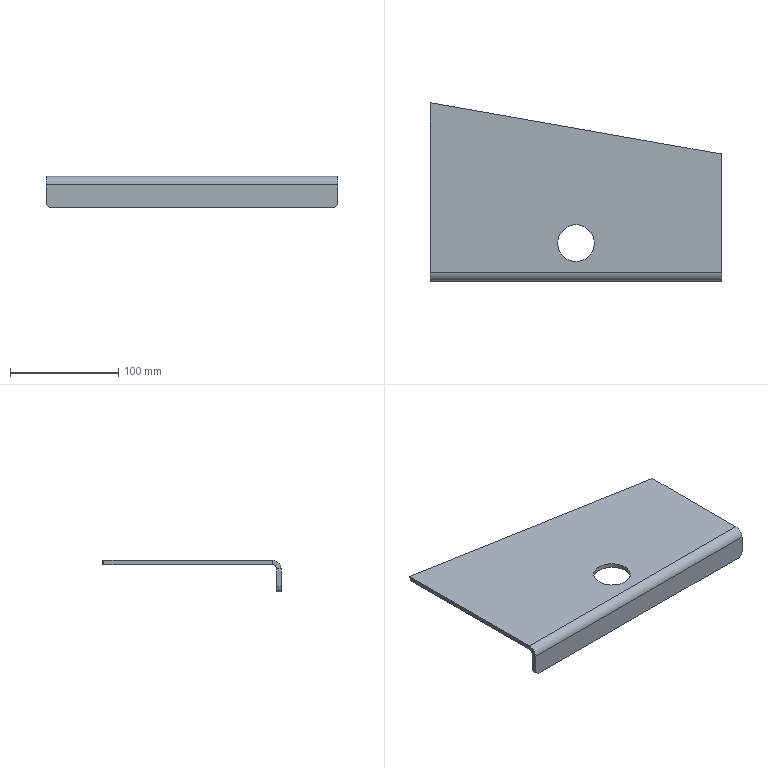Part | STEP file | 001-011-Blanking flip vertical plate | 1 solid | 20 faces | box 270 x 164.808 x 29 mm | volume 173034 mm3 | plane 12 | cylinder 8 | commonest cylinder face diameters 2 x2 10 x2 34 x2 8 x1 16 x1
STEP:
#1=CARTESIAN_POINT('',(0.,0.,0.));
#2=DIRECTION('',(0.,0.,1.));
#3=DIRECTION('',(1.,0.,0.));
#4=AXIS2_PLACEMENT_3D('',#1,#2,#3);
#5=CARTESIAN_POINT('',(-17.,-47.5,0.));
#6=VERTEX_POINT('',#5);
#7=CARTESIAN_POINT('',(-17.,-47.5,-4.));
#8=VERTEX_POINT('',#7);
#9=CARTESIAN_POINT('',(-17.,-47.5,0.));
#10=DIRECTION('',(0.,0.,-1.));
#11=VECTOR('',#10,1.);
#12=LINE('',#9,#11);
#13=CARTESIAN_POINT('',(0.,-47.5,0.));
#14=DIRECTION('',(0.,0.,-1.));
#15=DIRECTION('',(-1.,0.,0.));
#16=AXIS2_PLACEMENT_3D('',#13,#14,#15);
#17=CYLINDRICAL_SURFACE('',#16,17.);
#18=CARTESIAN_POINT('',(6.283,0.));
#19=DIRECTION('',(0.,1.));
#20=VECTOR('',#19,1.);
#21=LINE('',#18,#20);
#22=(GEOMETRIC_REPRESENTATION_CONTEXT(2)PARAMETRIC_REPRESENTATION_CONTEXT()REPRESENTATION_CONTEXT('',''));
#23=DEFINITIONAL_REPRESENTATION('',(#21),#22);
#24=PCURVE('',#17,#23);
#25=CARTESIAN_POINT('',(0.,-47.5,0.));
#26=DIRECTION('',(0.,0.,-1.));
#27=DIRECTION('',(-1.,0.,0.));
#28=AXIS2_PLACEMENT_3D('',#25,#26,#27);
#29=CYLINDRICAL_SURFACE('',#28,17.);
#30=CARTESIAN_POINT('',(0.,0.));
#31=DIRECTION('',(0.,1.));
#32=VECTOR('',#31,1.);
#33=LINE('',#30,#32);
#34=(GEOMETRIC_REPRESENTATION_CONTEXT(2)PARAMETRIC_REPRESENTATION_CONTEXT()REPRESENTATION_CONTEXT('',''));
#35=DEFINITIONAL_REPRESENTATION('',(#33),#34);
#36=PCURVE('',#29,#35);
#37=SURFACE_CURVE('',#12,(#24,#36),.PCURVE_S1.);
#38=EDGE_CURVE('',#6,#8,#37,.T.);
#39=ORIENTED_EDGE('',*,*,#38,.T.);
#40=CARTESIAN_POINT('',(17.,-47.5,-4.));
#41=VERTEX_POINT('',#40);
#42=CARTESIAN_POINT('',(0.,-47.5,-4.));
#43=DIRECTION('',(0.,0.,-1.));
#44=DIRECTION('',(-1.,0.,0.));
#45=AXIS2_PLACEMENT_3D('',#42,#43,#44);
#46=CIRCLE('',#45,17.);
#47=CARTESIAN_POINT('',(0.,4.));
#48=DIRECTION('',(1.,0.));
#49=VECTOR('',#48,1.);
#50=LINE('',#47,#49);
#51=(GEOMETRIC_REPRESENTATION_CONTEXT(2)PARAMETRIC_REPRESENTATION_CONTEXT()REPRESENTATION_CONTEXT('',''));
#52=DEFINITIONAL_REPRESENTATION('',(#50),#51);
#53=PCURVE('',#17,#52);
#54=CARTESIAN_POINT('',(0.,0.,-4.));
#55=DIRECTION('',(0.,0.,-1.));
#56=DIRECTION('',(-1.,0.,0.));
#57=AXIS2_PLACEMENT_3D('',#54,#55,#56);
#58=PLANE('',#57);
#59=CARTESIAN_POINT('',(0.,-47.5));
#60=DIRECTION('',(1.,0.));
#61=AXIS2_PLACEMENT_2D('',#59,#60);
#62=CIRCLE('',#61,17.);
#63=(GEOMETRIC_REPRESENTATION_CONTEXT(2)PARAMETRIC_REPRESENTATION_CONTEXT()REPRESENTATION_CONTEXT('',''));
#64=DEFINITIONAL_REPRESENTATION('',(#62),#63);
#65=PCURVE('',#58,#64);
#66=SURFACE_CURVE('',#46,(#53,#65),.PCURVE_S1.);
#67=EDGE_CURVE('',#41,#8,#66,.T.);
#68=ORIENTED_EDGE('',*,*,#67,.F.);
#69=CARTESIAN_POINT('',(17.,-47.5,0.));
#70=VERTEX_POINT('',#69);
#71=CARTESIAN_POINT('',(17.,-47.5,0.));
#72=DIRECTION('',(0.,0.,-1.));
#73=VECTOR('',#72,1.);
#74=LINE('',#71,#73);
#75=CARTESIAN_POINT('',(3.142,0.));
#76=DIRECTION('',(0.,1.));
#77=VECTOR('',#76,1.);
#78=LINE('',#75,#77);
#79=(GEOMETRIC_REPRESENTATION_CONTEXT(2)PARAMETRIC_REPRESENTATION_CONTEXT()REPRESENTATION_CONTEXT('',''));
#80=DEFINITIONAL_REPRESENTATION('',(#78),#79);
#81=PCURVE('',#17,#80);
#82=CARTESIAN_POINT('',(3.142,0.));
#83=DIRECTION('',(0.,1.));
#84=VECTOR('',#83,1.);
#85=LINE('',#82,#84);
#86=(GEOMETRIC_REPRESENTATION_CONTEXT(2)PARAMETRIC_REPRESENTATION_CONTEXT()REPRESENTATION_CONTEXT('',''));
#87=DEFINITIONAL_REPRESENTATION('',(#85),#86);
#88=PCURVE('',#29,#87);
#89=SURFACE_CURVE('',#74,(#81,#88),.PCURVE_S1.);
#90=EDGE_CURVE('',#70,#41,#89,.T.);
#91=ORIENTED_EDGE('',*,*,#90,.F.);
#92=CARTESIAN_POINT('',(0.,-47.5,0.));
#93=DIRECTION('',(0.,0.,-1.));
#94=DIRECTION('',(-1.,0.,0.));
#95=AXIS2_PLACEMENT_3D('',#92,#93,#94);
#96=CIRCLE('',#95,17.);
#97=CARTESIAN_POINT('',(0.,0.));
#98=DIRECTION('',(1.,0.));
#99=VECTOR('',#98,1.);
#100=LINE('',#97,#99);
#101=(GEOMETRIC_REPRESENTATION_CONTEXT(2)PARAMETRIC_REPRESENTATION_CONTEXT()REPRESENTATION_CONTEXT('',''));
#102=DEFINITIONAL_REPRESENTATION('',(#100),#101);
#103=PCURVE('',#17,#102);
#104=CARTESIAN_POINT('',(0.,0.,0.));
#105=DIRECTION('',(0.,0.,-1.));
#106=DIRECTION('',(-1.,0.,0.));
#107=AXIS2_PLACEMENT_3D('',#104,#105,#106);
#108=PLANE('',#107);
#109=CARTESIAN_POINT('',(0.,-47.5));
#110=DIRECTION('',(1.,0.));
#111=AXIS2_PLACEMENT_2D('',#109,#110);
#112=CIRCLE('',#111,17.);
#113=(GEOMETRIC_REPRESENTATION_CONTEXT(2)PARAMETRIC_REPRESENTATION_CONTEXT()REPRESENTATION_CONTEXT('',''));
#114=DEFINITIONAL_REPRESENTATION('',(#112),#113);
#115=PCURVE('',#108,#114);
#116=SURFACE_CURVE('',#96,(#103,#115),.PCURVE_S1.);
#117=EDGE_CURVE('',#70,#6,#116,.T.);
#118=ORIENTED_EDGE('',*,*,#117,.T.);
#119=EDGE_LOOP('',(#39,#68,#91,#118));
#120=FACE_BOUND('',#119,.F.);
#121=ADVANCED_FACE('',(#120),#17,.F.);
#122=CARTESIAN_POINT('',(-135.,81.308,0.));
#123=VERTEX_POINT('',#122);
#124=CARTESIAN_POINT('',(-135.,-74.5,0.));
#125=VERTEX_POINT('',#124);
#126=CARTESIAN_POINT('',(-135.,-82.5,0.));
#127=DIRECTION('',(0.,-1.,0.));
#128=VECTOR('',#127,1.);
#129=LINE('',#126,#128);
#130=CARTESIAN_POINT('',(-135.,-82.5,-4.));
#131=DIRECTION('',(-1.,0.,0.));
#132=DIRECTION('',(0.,0.,1.));
#133=AXIS2_PLACEMENT_3D('',#130,#131,#132);
#134=PLANE('',#133);
#135=CARTESIAN_POINT('',(4.,0.));
#136=DIRECTION('',(0.,-1.));
#137=VECTOR('',#136,1.);
#138=LINE('',#135,#137);
#139=(GEOMETRIC_REPRESENTATION_CONTEXT(2)PARAMETRIC_REPRESENTATION_CONTEXT()REPRESENTATION_CONTEXT('',''));
#140=DEFINITIONAL_REPRESENTATION('',(#138),#139);
#141=PCURVE('',#134,#140);
#142=CARTESIAN_POINT('',(135.,-82.5));
#143=DIRECTION('',(0.,-1.));
#144=VECTOR('',#143,1.);
#145=LINE('',#142,#144);
#146=(GEOMETRIC_REPRESENTATION_CONTEXT(2)PARAMETRIC_REPRESENTATION_CONTEXT()REPRESENTATION_CONTEXT('',''));
#147=DEFINITIONAL_REPRESENTATION('',(#145),#146);
#148=PCURVE('',#108,#147);
#149=SURFACE_CURVE('',#129,(#141,#148),.PCURVE_S1.);
#150=EDGE_CURVE('',#123,#125,#149,.T.);
#151=ORIENTED_EDGE('',*,*,#150,.F.);
#152=CARTESIAN_POINT('',(-135.,81.308,-4.));
#153=VERTEX_POINT('',#152);
#154=CARTESIAN_POINT('',(-135.,81.308,-4.));
#155=DIRECTION('',(0.,0.,-1.));
#156=VECTOR('',#155,1.);
#157=LINE('',#154,#156);
#158=CARTESIAN_POINT('',(0.,163.808));
#159=DIRECTION('',(-1.,0.));
#160=VECTOR('',#159,1.);
#161=LINE('',#158,#160);
#162=(GEOMETRIC_REPRESENTATION_CONTEXT(2)PARAMETRIC_REPRESENTATION_CONTEXT()REPRESENTATION_CONTEXT('',''));
#163=DEFINITIONAL_REPRESENTATION('',(#161),#162);
#164=PCURVE('',#134,#163);
#165=CARTESIAN_POINT('',(-134.,81.308,-29.));
#166=DIRECTION('',(0.,0.,-1.));
#167=DIRECTION('',(-1.,0.,0.));
#168=AXIS2_PLACEMENT_3D('',#165,#166,#167);
#169=CYLINDRICAL_SURFACE('',#168,1.);
#170=CARTESIAN_POINT('',(0.,-25.));
#171=DIRECTION('',(0.,1.));
#172=VECTOR('',#171,1.);
#173=LINE('',#170,#172);
#174=(GEOMETRIC_REPRESENTATION_CONTEXT(2)PARAMETRIC_REPRESENTATION_CONTEXT()REPRESENTATION_CONTEXT('',''));
#175=DEFINITIONAL_REPRESENTATION('',(#173),#174);
#176=PCURVE('',#169,#175);
#177=SURFACE_CURVE('',#157,(#164,#176),.PCURVE_S1.);
#178=EDGE_CURVE('',#123,#153,#177,.T.);
#179=ORIENTED_EDGE('',*,*,#178,.T.);
#180=CARTESIAN_POINT('',(-135.,-74.5,-4.));
#181=VERTEX_POINT('',#180);
#182=CARTESIAN_POINT('',(-135.,-82.5,-4.));
#183=DIRECTION('',(0.,-1.,0.));
#184=VECTOR('',#183,1.);
#185=LINE('',#182,#184);
#186=CARTESIAN_POINT('',(0.,0.));
#187=DIRECTION('',(0.,-1.));
#188=VECTOR('',#187,1.);
#189=LINE('',#186,#188);
#190=(GEOMETRIC_REPRESENTATION_CONTEXT(2)PARAMETRIC_REPRESENTATION_CONTEXT()REPRESENTATION_CONTEXT('',''));
#191=DEFINITIONAL_REPRESENTATION('',(#189),#190);
#192=PCURVE('',#134,#191);
#193=CARTESIAN_POINT('',(135.,-82.5));
#194=DIRECTION('',(0.,-1.));
#195=VECTOR('',#194,1.);
#196=LINE('',#193,#195);
#197=(GEOMETRIC_REPRESENTATION_CONTEXT(2)PARAMETRIC_REPRESENTATION_CONTEXT()REPRESENTATION_CONTEXT('',''));
#198=DEFINITIONAL_REPRESENTATION('',(#196),#197);
#199=PCURVE('',#58,#198);
#200=SURFACE_CURVE('',#185,(#192,#199),.PCURVE_S1.);
#201=EDGE_CURVE('',#153,#181,#200,.T.);
#202=ORIENTED_EDGE('',*,*,#201,.T.);
#203=CARTESIAN_POINT('',(-135.,-74.5,-4.));
#204=DIRECTION('',(0.,0.,1.));
#205=VECTOR('',#204,1.);
#206=LINE('',#203,#205);
#207=CARTESIAN_POINT('',(0.,8.));
#208=DIRECTION('',(1.,0.));
#209=VECTOR('',#208,1.);
#210=LINE('',#207,#209);
#211=(GEOMETRIC_REPRESENTATION_CONTEXT(2)PARAMETRIC_REPRESENTATION_CONTEXT()REPRESENTATION_CONTEXT('',''));
#212=DEFINITIONAL_REPRESENTATION('',(#210),#211);
#213=PCURVE('',#134,#212);
#214=CARTESIAN_POINT('',(-135.,-74.5,-8.));
#215=DIRECTION('',(1.,0.,0.));
#216=DIRECTION('',(0.,0.,-1.));
#217=AXIS2_PLACEMENT_3D('',#214,#215,#216);
#218=PLANE('',#217);
#219=CARTESIAN_POINT('',(-4.,0.));
#220=DIRECTION('',(-1.,0.));
#221=VECTOR('',#220,1.);
#222=LINE('',#219,#221);
#223=(GEOMETRIC_REPRESENTATION_CONTEXT(2)PARAMETRIC_REPRESENTATION_CONTEXT()REPRESENTATION_CONTEXT('',''));
#224=DEFINITIONAL_REPRESENTATION('',(#222),#223);
#225=PCURVE('',#218,#224);
#226=SURFACE_CURVE('',#206,(#213,#225),.PCURVE_S1.);
#227=EDGE_CURVE('',#181,#125,#226,.T.);
#228=ORIENTED_EDGE('',*,*,#227,.T.);
#229=EDGE_LOOP('',(#151,#179,#202,#228));
#230=FACE_BOUND('',#229,.T.);
#231=ADVANCED_FACE('',(#230),#134,.T.);
#232=CARTESIAN_POINT('',(0.,-47.5,-4.));
#233=DIRECTION('',(0.,0.,-1.));
#234=DIRECTION('',(-1.,0.,0.));
#235=AXIS2_PLACEMENT_3D('',#232,#233,#234);
#236=CIRCLE('',#235,17.);
#237=CARTESIAN_POINT('',(0.,-47.5));
#238=DIRECTION('',(1.,0.));
#239=AXIS2_PLACEMENT_2D('',#237,#238);
#240=CIRCLE('',#239,17.);
#241=(GEOMETRIC_REPRESENTATION_CONTEXT(2)PARAMETRIC_REPRESENTATION_CONTEXT()REPRESENTATION_CONTEXT('',''));
#242=DEFINITIONAL_REPRESENTATION('',(#240),#241);
#243=PCURVE('',#58,#242);
#244=CARTESIAN_POINT('',(0.,4.));
#245=DIRECTION('',(1.,0.));
#246=VECTOR('',#245,1.);
#247=LINE('',#244,#246);
#248=(GEOMETRIC_REPRESENTATION_CONTEXT(2)PARAMETRIC_REPRESENTATION_CONTEXT()REPRESENTATION_CONTEXT('',''));
#249=DEFINITIONAL_REPRESENTATION('',(#247),#248);
#250=PCURVE('',#29,#249);
#251=SURFACE_CURVE('',#236,(#243,#250),.PCURVE_S1.);
#252=EDGE_CURVE('',#8,#41,#251,.T.);
#253=ORIENTED_EDGE('',*,*,#252,.F.);
#254=ORIENTED_EDGE('',*,*,#67,.F.);
#255=EDGE_LOOP('',(#253,#254));
#256=FACE_BOUND('',#255,.T.);
#257=ORIENTED_EDGE('',*,*,#201,.F.);
#258=CARTESIAN_POINT('',(-133.826,82.293,-4.));
#259=VERTEX_POINT('',#258);
#260=CARTESIAN_POINT('',(-134.,81.308,-4.));
#261=DIRECTION('',(0.,0.,-1.));
#262=DIRECTION('',(-1.,0.,0.));
#263=AXIS2_PLACEMENT_3D('',#260,#261,#262);
#264=CIRCLE('',#263,1.);
#265=CARTESIAN_POINT('',(134.,81.308));
#266=DIRECTION('',(1.,0.));
#267=AXIS2_PLACEMENT_2D('',#265,#266);
#268=CIRCLE('',#267,1.);
#269=(GEOMETRIC_REPRESENTATION_CONTEXT(2)PARAMETRIC_REPRESENTATION_CONTEXT()REPRESENTATION_CONTEXT('',''));
#270=DEFINITIONAL_REPRESENTATION('',(#268),#269);
#271=PCURVE('',#58,#270);
#272=CARTESIAN_POINT('',(0.,-25.));
#273=DIRECTION('',(1.,0.));
#274=VECTOR('',#273,1.);
#275=LINE('',#272,#274);
#276=(GEOMETRIC_REPRESENTATION_CONTEXT(2)PARAMETRIC_REPRESENTATION_CONTEXT()REPRESENTATION_CONTEXT('',''));
#277=DEFINITIONAL_REPRESENTATION('',(#275),#276);
#278=PCURVE('',#169,#277);
#279=SURFACE_CURVE('',#264,(#271,#278),.PCURVE_S1.);
#280=EDGE_CURVE('',#153,#259,#279,.T.);
#281=ORIENTED_EDGE('',*,*,#280,.T.);
#282=CARTESIAN_POINT('',(134.174,35.037,-4.));
#283=VERTEX_POINT('',#282);
#284=CARTESIAN_POINT('',(10.038,56.926,-4.));
#285=DIRECTION('',(-0.9848,0.1736,0.));
#286=VECTOR('',#285,1.);
#287=LINE('',#284,#286);
#288=CARTESIAN_POINT('',(-10.038,56.926));
#289=DIRECTION('',(0.9848,0.1736));
#290=VECTOR('',#289,1.);
#291=LINE('',#288,#290);
#292=(GEOMETRIC_REPRESENTATION_CONTEXT(2)PARAMETRIC_REPRESENTATION_CONTEXT()REPRESENTATION_CONTEXT('',''));
#293=DEFINITIONAL_REPRESENTATION('',(#291),#292);
#294=PCURVE('',#58,#293);
#295=CARTESIAN_POINT('',(135.,34.892,-29.));
#296=DIRECTION('',(-0.1736,-0.9848,0.));
#297=DIRECTION('',(0.9848,-0.1736,0.));
#298=AXIS2_PLACEMENT_3D('',#295,#296,#297);
#299=PLANE('',#298);
#300=CARTESIAN_POINT('',(-126.89,25.));
#301=DIRECTION('',(-1.,0.));
#302=VECTOR('',#301,1.);
#303=LINE('',#300,#302);
#304=(GEOMETRIC_REPRESENTATION_CONTEXT(2)PARAMETRIC_REPRESENTATION_CONTEXT()REPRESENTATION_CONTEXT('',''));
#305=DEFINITIONAL_REPRESENTATION('',(#303),#304);
#306=PCURVE('',#299,#305);
#307=SURFACE_CURVE('',#287,(#294,#306),.PCURVE_S1.);
#308=EDGE_CURVE('',#283,#259,#307,.T.);
#309=ORIENTED_EDGE('',*,*,#308,.F.);
#310=CARTESIAN_POINT('',(135.,34.053,-4.));
#311=VERTEX_POINT('',#310);
#312=CARTESIAN_POINT('',(134.,34.053,-4.));
#313=DIRECTION('',(0.,0.,-1.));
#314=DIRECTION('',(-1.,0.,0.));
#315=AXIS2_PLACEMENT_3D('',#312,#313,#314);
#316=CIRCLE('',#315,1.);
#317=CARTESIAN_POINT('',(-134.,34.053));
#318=DIRECTION('',(1.,0.));
#319=AXIS2_PLACEMENT_2D('',#317,#318);
#320=CIRCLE('',#319,1.);
#321=(GEOMETRIC_REPRESENTATION_CONTEXT(2)PARAMETRIC_REPRESENTATION_CONTEXT()REPRESENTATION_CONTEXT('',''));
#322=DEFINITIONAL_REPRESENTATION('',(#320),#321);
#323=PCURVE('',#58,#322);
#324=CARTESIAN_POINT('',(134.,34.053,-4.));
#325=DIRECTION('',(0.,0.,-1.));
#326=DIRECTION('',(-1.,0.,0.));
#327=AXIS2_PLACEMENT_3D('',#324,#325,#326);
#328=CYLINDRICAL_SURFACE('',#327,1.);
#329=CARTESIAN_POINT('',(0.,0.));
#330=DIRECTION('',(1.,0.));
#331=VECTOR('',#330,1.);
#332=LINE('',#329,#331);
#333=(GEOMETRIC_REPRESENTATION_CONTEXT(2)PARAMETRIC_REPRESENTATION_CONTEXT()REPRESENTATION_CONTEXT('',''));
#334=DEFINITIONAL_REPRESENTATION('',(#332),#333);
#335=PCURVE('',#328,#334);
#336=SURFACE_CURVE('',#316,(#323,#335),.PCURVE_S1.);
#337=EDGE_CURVE('',#283,#311,#336,.T.);
#338=ORIENTED_EDGE('',*,*,#337,.T.);
#339=CARTESIAN_POINT('',(135.,-74.5,-4.));
#340=VERTEX_POINT('',#339);
#341=CARTESIAN_POINT('',(135.,-82.5,-4.));
#342=DIRECTION('',(0.,1.,0.));
#343=VECTOR('',#342,1.);
#344=LINE('',#341,#343);
#345=CARTESIAN_POINT('',(-135.,-82.5));
#346=DIRECTION('',(0.,1.));
#347=VECTOR('',#346,1.);
#348=LINE('',#345,#347);
#349=(GEOMETRIC_REPRESENTATION_CONTEXT(2)PARAMETRIC_REPRESENTATION_CONTEXT()REPRESENTATION_CONTEXT('',''));
#350=DEFINITIONAL_REPRESENTATION('',(#348),#349);
#351=PCURVE('',#58,#350);
#352=CARTESIAN_POINT('',(135.,-82.5,-4.));
#353=DIRECTION('',(1.,0.,0.));
#354=DIRECTION('',(0.,1.,0.));
#355=AXIS2_PLACEMENT_3D('',#352,#353,#354);
#356=PLANE('',#355);
#357=CARTESIAN_POINT('',(0.,0.));
#358=DIRECTION('',(1.,0.));
#359=VECTOR('',#358,1.);
#360=LINE('',#357,#359);
#361=(GEOMETRIC_REPRESENTATION_CONTEXT(2)PARAMETRIC_REPRESENTATION_CONTEXT()REPRESENTATION_CONTEXT('',''));
#362=DEFINITIONAL_REPRESENTATION('',(#360),#361);
#363=PCURVE('',#356,#362);
#364=SURFACE_CURVE('',#344,(#351,#363),.PCURVE_S1.);
#365=EDGE_CURVE('',#340,#311,#364,.T.);
#366=ORIENTED_EDGE('',*,*,#365,.F.);
#367=CARTESIAN_POINT('',(-135.,-74.5,-4.));
#368=DIRECTION('',(1.,0.,0.));
#369=VECTOR('',#368,1.);
#370=LINE('',#367,#369);
#371=CARTESIAN_POINT('',(135.,-74.5));
#372=DIRECTION('',(-1.,0.));
#373=VECTOR('',#372,1.);
#374=LINE('',#371,#373);
#375=(GEOMETRIC_REPRESENTATION_CONTEXT(2)PARAMETRIC_REPRESENTATION_CONTEXT()REPRESENTATION_CONTEXT('',''));
#376=DEFINITIONAL_REPRESENTATION('',(#374),#375);
#377=PCURVE('',#58,#376);
#378=CARTESIAN_POINT('',(-135.,-74.5,-8.));
#379=DIRECTION('',(-1.,0.,0.));
#380=DIRECTION('',(0.,-1.,0.));
#381=AXIS2_PLACEMENT_3D('',#378,#379,#380);
#382=CYLINDRICAL_SURFACE('',#381,4.);
#383=CARTESIAN_POINT('',(1.571,0.));
#384=DIRECTION('',(0.,-1.));
#385=VECTOR('',#384,1.);
#386=LINE('',#383,#385);
#387=(GEOMETRIC_REPRESENTATION_CONTEXT(2)PARAMETRIC_REPRESENTATION_CONTEXT()REPRESENTATION_CONTEXT('',''));
#388=DEFINITIONAL_REPRESENTATION('',(#386),#387);
#389=PCURVE('',#382,#388);
#390=SURFACE_CURVE('',#370,(#377,#389),.PCURVE_S1.);
#391=EDGE_CURVE('',#181,#340,#390,.T.);
#392=ORIENTED_EDGE('',*,*,#391,.F.);
#393=EDGE_LOOP('',(#257,#281,#309,#338,#366,#392));
#394=FACE_BOUND('',#393,.T.);
#395=ADVANCED_FACE('',(#256,#394),#58,.T.);
#396=CARTESIAN_POINT('',(0.,-47.5,0.));
#397=DIRECTION('',(0.,0.,-1.));
#398=DIRECTION('',(-1.,0.,0.));
#399=AXIS2_PLACEMENT_3D('',#396,#397,#398);
#400=CIRCLE('',#399,17.);
#401=CARTESIAN_POINT('',(0.,-47.5));
#402=DIRECTION('',(1.,0.));
#403=AXIS2_PLACEMENT_2D('',#401,#402);
#404=CIRCLE('',#403,17.);
#405=(GEOMETRIC_REPRESENTATION_CONTEXT(2)PARAMETRIC_REPRESENTATION_CONTEXT()REPRESENTATION_CONTEXT('',''));
#406=DEFINITIONAL_REPRESENTATION('',(#404),#405);
#407=PCURVE('',#108,#406);
#408=CARTESIAN_POINT('',(0.,0.));
#409=DIRECTION('',(1.,0.));
#410=VECTOR('',#409,1.);
#411=LINE('',#408,#410);
#412=(GEOMETRIC_REPRESENTATION_CONTEXT(2)PARAMETRIC_REPRESENTATION_CONTEXT()REPRESENTATION_CONTEXT('',''));
#413=DEFINITIONAL_REPRESENTATION('',(#411),#412);
#414=PCURVE('',#29,#413);
#415=SURFACE_CURVE('',#400,(#407,#414),.PCURVE_S1.);
#416=EDGE_CURVE('',#6,#70,#415,.T.);
#417=ORIENTED_EDGE('',*,*,#416,.T.);
#418=ORIENTED_EDGE('',*,*,#117,.T.);
#419=EDGE_LOOP('',(#417,#418));
#420=FACE_BOUND('',#419,.T.);
#421=CARTESIAN_POINT('',(-133.826,82.293,0.));
#422=VERTEX_POINT('',#421);
#423=CARTESIAN_POINT('',(134.174,35.037,0.));
#424=VERTEX_POINT('',#423);
#425=CARTESIAN_POINT('',(135.,34.892,0.));
#426=DIRECTION('',(0.9848,-0.1736,0.));
#427=VECTOR('',#426,1.);
#428=LINE('',#425,#427);
#429=CARTESIAN_POINT('',(-135.,34.892));
#430=DIRECTION('',(-0.9848,-0.1736));
#431=VECTOR('',#430,1.);
#432=LINE('',#429,#431);
#433=(GEOMETRIC_REPRESENTATION_CONTEXT(2)PARAMETRIC_REPRESENTATION_CONTEXT()REPRESENTATION_CONTEXT('',''));
#434=DEFINITIONAL_REPRESENTATION('',(#432),#433);
#435=PCURVE('',#108,#434);
#436=CARTESIAN_POINT('',(0.,29.));
#437=DIRECTION('',(1.,0.));
#438=VECTOR('',#437,1.);
#439=LINE('',#436,#438);
#440=(GEOMETRIC_REPRESENTATION_CONTEXT(2)PARAMETRIC_REPRESENTATION_CONTEXT()REPRESENTATION_CONTEXT('',''));
#441=DEFINITIONAL_REPRESENTATION('',(#439),#440);
#442=PCURVE('',#299,#441);
#443=SURFACE_CURVE('',#428,(#435,#442),.PCURVE_S1.);
#444=EDGE_CURVE('',#422,#424,#443,.T.);
#445=ORIENTED_EDGE('',*,*,#444,.F.);
#446=CARTESIAN_POINT('',(-134.,81.308,0.));
#447=DIRECTION('',(0.,0.,1.));
#448=DIRECTION('',(-1.,0.,0.));
#449=AXIS2_PLACEMENT_3D('',#446,#447,#448);
#450=CIRCLE('',#449,1.);
#451=CARTESIAN_POINT('',(135.,81.308));
#452=CARTESIAN_POINT('',(135.,79.576));
#453=CARTESIAN_POINT('',(133.5,80.442));
#454=CARTESIAN_POINT('',(132.,81.308));
#455=CARTESIAN_POINT('',(133.5,82.174));
#456=CARTESIAN_POINT('',(135.,83.04));
#457=CARTESIAN_POINT('',(135.,81.308));
#458=(BOUNDED_CURVE()B_SPLINE_CURVE(2,(#451,#452,#453,#454,#455,#456,#457),.UNSPECIFIED.,.T.,.F.)B_SPLINE_CURVE_WITH_KNOTS((1,2,2,2,2,1),(-2.094,0.,2.094,4.189,6.283,8.378),.UNSPECIFIED.)CURVE()GEOMETRIC_REPRESENTATION_ITEM()RATIONAL_B_SPLINE_CURVE((1.,0.5,1.,0.5,1.,0.5,1.))REPRESENTATION_ITEM(''));
#459=(GEOMETRIC_REPRESENTATION_CONTEXT(2)PARAMETRIC_REPRESENTATION_CONTEXT()REPRESENTATION_CONTEXT('',''));
#460=DEFINITIONAL_REPRESENTATION('',(#458),#459);
#461=PCURVE('',#108,#460);
#462=CARTESIAN_POINT('',(6.283,-29.));
#463=DIRECTION('',(-1.,0.));
#464=VECTOR('',#463,1.);
#465=LINE('',#462,#464);
#466=(GEOMETRIC_REPRESENTATION_CONTEXT(2)PARAMETRIC_REPRESENTATION_CONTEXT()REPRESENTATION_CONTEXT('',''));
#467=DEFINITIONAL_REPRESENTATION('',(#465),#466);
#468=PCURVE('',#169,#467);
#469=SURFACE_CURVE('',#450,(#461,#468),.PCURVE_S1.);
#470=EDGE_CURVE('',#422,#123,#469,.T.);
#471=ORIENTED_EDGE('',*,*,#470,.T.);
#472=ORIENTED_EDGE('',*,*,#150,.T.);
#473=CARTESIAN_POINT('',(135.,-74.5,0.));
#474=VERTEX_POINT('',#473);
#475=CARTESIAN_POINT('',(-135.,-74.5,0.));
#476=DIRECTION('',(1.,0.,0.));
#477=VECTOR('',#476,1.);
#478=LINE('',#475,#477);
#479=CARTESIAN_POINT('',(135.,-74.5));
#480=DIRECTION('',(-1.,0.));
#481=VECTOR('',#480,1.);
#482=LINE('',#479,#481);
#483=(GEOMETRIC_REPRESENTATION_CONTEXT(2)PARAMETRIC_REPRESENTATION_CONTEXT()REPRESENTATION_CONTEXT('',''));
#484=DEFINITIONAL_REPRESENTATION('',(#482),#483);
#485=PCURVE('',#108,#484);
#486=CARTESIAN_POINT('',(-135.,-74.5,-8.));
#487=DIRECTION('',(-1.,0.,0.));
#488=DIRECTION('',(0.,-1.,0.));
#489=AXIS2_PLACEMENT_3D('',#486,#487,#488);
#490=CYLINDRICAL_SURFACE('',#489,8.);
#491=CARTESIAN_POINT('',(1.571,0.));
#492=DIRECTION('',(0.,-1.));
#493=VECTOR('',#492,1.);
#494=LINE('',#491,#493);
#495=(GEOMETRIC_REPRESENTATION_CONTEXT(2)PARAMETRIC_REPRESENTATION_CONTEXT()REPRESENTATION_CONTEXT('',''));
#496=DEFINITIONAL_REPRESENTATION('',(#494),#495);
#497=PCURVE('',#490,#496);
#498=SURFACE_CURVE('',#478,(#485,#497),.PCURVE_S1.);
#499=EDGE_CURVE('',#125,#474,#498,.T.);
#500=ORIENTED_EDGE('',*,*,#499,.T.);
#501=CARTESIAN_POINT('',(135.,34.053,0.));
#502=VERTEX_POINT('',#501);
#503=CARTESIAN_POINT('',(135.,-82.5,0.));
#504=DIRECTION('',(0.,1.,0.));
#505=VECTOR('',#504,1.);
#506=LINE('',#503,#505);
#507=CARTESIAN_POINT('',(-135.,-82.5));
#508=DIRECTION('',(0.,1.));
#509=VECTOR('',#508,1.);
#510=LINE('',#507,#509);
#511=(GEOMETRIC_REPRESENTATION_CONTEXT(2)PARAMETRIC_REPRESENTATION_CONTEXT()REPRESENTATION_CONTEXT('',''));
#512=DEFINITIONAL_REPRESENTATION('',(#510),#511);
#513=PCURVE('',#108,#512);
#514=CARTESIAN_POINT('',(0.,4.));
#515=DIRECTION('',(1.,0.));
#516=VECTOR('',#515,1.);
#517=LINE('',#514,#516);
#518=(GEOMETRIC_REPRESENTATION_CONTEXT(2)PARAMETRIC_REPRESENTATION_CONTEXT()REPRESENTATION_CONTEXT('',''));
#519=DEFINITIONAL_REPRESENTATION('',(#517),#518);
#520=PCURVE('',#356,#519);
#521=SURFACE_CURVE('',#506,(#513,#520),.PCURVE_S1.);
#522=EDGE_CURVE('',#474,#502,#521,.T.);
#523=ORIENTED_EDGE('',*,*,#522,.T.);
#524=CARTESIAN_POINT('',(134.,34.053,0.));
#525=DIRECTION('',(0.,0.,1.));
#526=DIRECTION('',(-1.,0.,0.));
#527=AXIS2_PLACEMENT_3D('',#524,#525,#526);
#528=CIRCLE('',#527,1.);
#529=CARTESIAN_POINT('',(-133.,34.053));
#530=CARTESIAN_POINT('',(-133.,32.321));
#531=CARTESIAN_POINT('',(-134.5,33.187));
#532=CARTESIAN_POINT('',(-136.,34.053));
#533=CARTESIAN_POINT('',(-134.5,34.919));
#534=CARTESIAN_POINT('',(-133.,35.785));
#535=CARTESIAN_POINT('',(-133.,34.053));
#536=(BOUNDED_CURVE()B_SPLINE_CURVE(2,(#529,#530,#531,#532,#533,#534,#535),.UNSPECIFIED.,.T.,.F.)B_SPLINE_CURVE_WITH_KNOTS((1,2,2,2,2,1),(-2.094,0.,2.094,4.189,6.283,8.378),.UNSPECIFIED.)CURVE()GEOMETRIC_REPRESENTATION_ITEM()RATIONAL_B_SPLINE_CURVE((1.,0.5,1.,0.5,1.,0.5,1.))REPRESENTATION_ITEM(''));
#537=(GEOMETRIC_REPRESENTATION_CONTEXT(2)PARAMETRIC_REPRESENTATION_CONTEXT()REPRESENTATION_CONTEXT('',''));
#538=DEFINITIONAL_REPRESENTATION('',(#536),#537);
#539=PCURVE('',#108,#538);
#540=CARTESIAN_POINT('',(6.283,-4.));
#541=DIRECTION('',(-1.,0.));
#542=VECTOR('',#541,1.);
#543=LINE('',#540,#542);
#544=(GEOMETRIC_REPRESENTATION_CONTEXT(2)PARAMETRIC_REPRESENTATION_CONTEXT()REPRESENTATION_CONTEXT('',''));
#545=DEFINITIONAL_REPRESENTATION('',(#543),#544);
#546=PCURVE('',#328,#545);
#547=SURFACE_CURVE('',#528,(#539,#546),.PCURVE_S1.);
#548=EDGE_CURVE('',#502,#424,#547,.T.);
#549=ORIENTED_EDGE('',*,*,#548,.T.);
#550=EDGE_LOOP('',(#445,#471,#472,#500,#523,#549));
#551=FACE_BOUND('',#550,.T.);
#552=ADVANCED_FACE('',(#420,#551),#108,.F.);
#553=ORIENTED_EDGE('',*,*,#365,.T.);
#554=CARTESIAN_POINT('',(135.,34.053,0.));
#555=DIRECTION('',(0.,0.,1.));
#556=VECTOR('',#555,1.);
#557=LINE('',#554,#556);
#558=CARTESIAN_POINT('',(116.553,4.));
#559=DIRECTION('',(0.,1.));
#560=VECTOR('',#559,1.);
#561=LINE('',#558,#560);
#562=(GEOMETRIC_REPRESENTATION_CONTEXT(2)PARAMETRIC_REPRESENTATION_CONTEXT()REPRESENTATION_CONTEXT('',''));
#563=DEFINITIONAL_REPRESENTATION('',(#561),#562);
#564=PCURVE('',#356,#563);
#565=CARTESIAN_POINT('',(3.142,-4.));
#566=DIRECTION('',(0.,-1.));
#567=VECTOR('',#566,1.);
#568=LINE('',#565,#567);
#569=(GEOMETRIC_REPRESENTATION_CONTEXT(2)PARAMETRIC_REPRESENTATION_CONTEXT()REPRESENTATION_CONTEXT('',''));
#570=DEFINITIONAL_REPRESENTATION('',(#568),#569);
#571=PCURVE('',#328,#570);
#572=SURFACE_CURVE('',#557,(#564,#571),.PCURVE_S1.);
#573=EDGE_CURVE('',#311,#502,#572,.T.);
#574=ORIENTED_EDGE('',*,*,#573,.T.);
#575=ORIENTED_EDGE('',*,*,#522,.F.);
#576=CARTESIAN_POINT('',(135.,-74.5,-4.));
#577=DIRECTION('',(0.,0.,1.));
#578=VECTOR('',#577,1.);
#579=LINE('',#576,#578);
#580=CARTESIAN_POINT('',(8.,0.));
#581=DIRECTION('',(0.,1.));
#582=VECTOR('',#581,1.);
#583=LINE('',#580,#582);
#584=(GEOMETRIC_REPRESENTATION_CONTEXT(2)PARAMETRIC_REPRESENTATION_CONTEXT()REPRESENTATION_CONTEXT('',''));
#585=DEFINITIONAL_REPRESENTATION('',(#583),#584);
#586=PCURVE('',#356,#585);
#587=CARTESIAN_POINT('',(135.,-74.5,-8.));
#588=DIRECTION('',(1.,0.,0.));
#589=DIRECTION('',(0.,0.,-1.));
#590=AXIS2_PLACEMENT_3D('',#587,#588,#589);
#591=PLANE('',#590);
#592=CARTESIAN_POINT('',(-4.,0.));
#593=DIRECTION('',(-1.,0.));
#594=VECTOR('',#593,1.);
#595=LINE('',#592,#594);
#596=(GEOMETRIC_REPRESENTATION_CONTEXT(2)PARAMETRIC_REPRESENTATION_CONTEXT()REPRESENTATION_CONTEXT('',''));
#597=DEFINITIONAL_REPRESENTATION('',(#595),#596);
#598=PCURVE('',#591,#597);
#599=SURFACE_CURVE('',#579,(#586,#598),.PCURVE_S1.);
#600=EDGE_CURVE('',#340,#474,#599,.T.);
#601=ORIENTED_EDGE('',*,*,#600,.F.);
#602=EDGE_LOOP('',(#553,#574,#575,#601));
#603=FACE_BOUND('',#602,.T.);
#604=ADVANCED_FACE('',(#603),#356,.T.);
#605=CARTESIAN_POINT('',(135.,-78.5,-8.));
#606=VERTEX_POINT('',#605);
#607=CARTESIAN_POINT('',(135.,-82.5,-8.));
#608=VERTEX_POINT('',#607);
#609=CARTESIAN_POINT('',(135.,-82.5,-8.));
#610=DIRECTION('',(0.,-1.,0.));
#611=VECTOR('',#610,1.);
#612=LINE('',#609,#611);
#613=CARTESIAN_POINT('',(0.,-8.));
#614=DIRECTION('',(0.,-1.));
#615=VECTOR('',#614,1.);
#616=LINE('',#613,#615);
#617=(GEOMETRIC_REPRESENTATION_CONTEXT(2)PARAMETRIC_REPRESENTATION_CONTEXT()REPRESENTATION_CONTEXT('',''));
#618=DEFINITIONAL_REPRESENTATION('',(#616),#617);
#619=PCURVE('',#591,#618);
#620=CARTESIAN_POINT('',(135.,-82.5,-29.));
#621=DIRECTION('',(1.,0.,0.));
#622=DIRECTION('',(0.,1.,0.));
#623=AXIS2_PLACEMENT_3D('',#620,#621,#622);
#624=PLANE('',#623);
#625=CARTESIAN_POINT('',(0.,21.));
#626=DIRECTION('',(-1.,0.));
#627=VECTOR('',#626,1.);
#628=LINE('',#625,#627);
#629=(GEOMETRIC_REPRESENTATION_CONTEXT(2)PARAMETRIC_REPRESENTATION_CONTEXT()REPRESENTATION_CONTEXT('',''));
#630=DEFINITIONAL_REPRESENTATION('',(#628),#629);
#631=PCURVE('',#624,#630);
#632=SURFACE_CURVE('',#612,(#619,#631),.PCURVE_S1.);
#633=EDGE_CURVE('',#606,#608,#632,.T.);
#634=ORIENTED_EDGE('',*,*,#633,.F.);
#635=CARTESIAN_POINT('',(135.,-74.5,-8.));
#636=DIRECTION('',(1.,0.,0.));
#637=DIRECTION('',(0.,0.,1.));
#638=AXIS2_PLACEMENT_3D('',#635,#636,#637);
#639=CIRCLE('',#638,4.);
#640=CARTESIAN_POINT('',(0.,0.));
#641=DIRECTION('',(-1.,0.));
#642=AXIS2_PLACEMENT_2D('',#640,#641);
#643=CIRCLE('',#642,4.);
#644=(GEOMETRIC_REPRESENTATION_CONTEXT(2)PARAMETRIC_REPRESENTATION_CONTEXT()REPRESENTATION_CONTEXT('',''));
#645=DEFINITIONAL_REPRESENTATION('',(#643),#644);
#646=PCURVE('',#591,#645);
#647=CARTESIAN_POINT('',(1.571,-270.));
#648=DIRECTION('',(-1.,0.));
#649=VECTOR('',#648,1.);
#650=LINE('',#647,#649);
#651=(GEOMETRIC_REPRESENTATION_CONTEXT(2)PARAMETRIC_REPRESENTATION_CONTEXT()REPRESENTATION_CONTEXT('',''));
#652=DEFINITIONAL_REPRESENTATION('',(#650),#651);
#653=PCURVE('',#382,#652);
#654=SURFACE_CURVE('',#639,(#646,#653),.PCURVE_S1.);
#655=EDGE_CURVE('',#340,#606,#654,.T.);
#656=ORIENTED_EDGE('',*,*,#655,.F.);
#657=ORIENTED_EDGE('',*,*,#600,.T.);
#658=CARTESIAN_POINT('',(135.,-74.5,-8.));
#659=DIRECTION('',(1.,0.,0.));
#660=DIRECTION('',(0.,0.,1.));
#661=AXIS2_PLACEMENT_3D('',#658,#659,#660);
#662=CIRCLE('',#661,8.);
#663=CARTESIAN_POINT('',(0.,0.));
#664=DIRECTION('',(-1.,0.));
#665=AXIS2_PLACEMENT_2D('',#663,#664);
#666=CIRCLE('',#665,8.);
#667=(GEOMETRIC_REPRESENTATION_CONTEXT(2)PARAMETRIC_REPRESENTATION_CONTEXT()REPRESENTATION_CONTEXT('',''));
#668=DEFINITIONAL_REPRESENTATION('',(#666),#667);
#669=PCURVE('',#591,#668);
#670=CARTESIAN_POINT('',(1.571,-270.));
#671=DIRECTION('',(-1.,0.));
#672=VECTOR('',#671,1.);
#673=LINE('',#670,#672);
#674=(GEOMETRIC_REPRESENTATION_CONTEXT(2)PARAMETRIC_REPRESENTATION_CONTEXT()REPRESENTATION_CONTEXT('',''));
#675=DEFINITIONAL_REPRESENTATION('',(#673),#674);
#676=PCURVE('',#490,#675);
#677=SURFACE_CURVE('',#662,(#669,#676),.PCURVE_S1.);
#678=EDGE_CURVE('',#474,#608,#677,.T.);
#679=ORIENTED_EDGE('',*,*,#678,.T.);
#680=EDGE_LOOP('',(#634,#656,#657,#679));
#681=FACE_BOUND('',#680,.T.);
#682=ADVANCED_FACE('',(#681),#591,.T.);
#683=CARTESIAN_POINT('',(-135.,-78.5,-8.));
#684=VERTEX_POINT('',#683);
#685=CARTESIAN_POINT('',(-135.,-74.5,-8.));
#686=DIRECTION('',(-1.,0.,0.));
#687=DIRECTION('',(0.,0.,1.));
#688=AXIS2_PLACEMENT_3D('',#685,#686,#687);
#689=CIRCLE('',#688,4.);
#690=CARTESIAN_POINT('',(-4.,0.));
#691=CARTESIAN_POINT('',(-4.,6.928));
#692=CARTESIAN_POINT('',(2.,3.464));
#693=CARTESIAN_POINT('',(8.,0.));
#694=CARTESIAN_POINT('',(2.,-3.464));
#695=CARTESIAN_POINT('',(-4.,-6.928));
#696=CARTESIAN_POINT('',(-4.,0.));
#697=(BOUNDED_CURVE()B_SPLINE_CURVE(2,(#690,#691,#692,#693,#694,#695,#696),.UNSPECIFIED.,.T.,.F.)B_SPLINE_CURVE_WITH_KNOTS((1,2,2,2,2,1),(-2.094,0.,2.094,4.189,6.283,8.378),.UNSPECIFIED.)CURVE()GEOMETRIC_REPRESENTATION_ITEM()RATIONAL_B_SPLINE_CURVE((1.,0.5,1.,0.5,1.,0.5,1.))REPRESENTATION_ITEM(''));
#698=(GEOMETRIC_REPRESENTATION_CONTEXT(2)PARAMETRIC_REPRESENTATION_CONTEXT()REPRESENTATION_CONTEXT('',''));
#699=DEFINITIONAL_REPRESENTATION('',(#697),#698);
#700=PCURVE('',#218,#699);
#701=CARTESIAN_POINT('',(-4.712,0.));
#702=DIRECTION('',(1.,0.));
#703=VECTOR('',#702,1.);
#704=LINE('',#701,#703);
#705=(GEOMETRIC_REPRESENTATION_CONTEXT(2)PARAMETRIC_REPRESENTATION_CONTEXT()REPRESENTATION_CONTEXT('',''));
#706=DEFINITIONAL_REPRESENTATION('',(#704),#705);
#707=PCURVE('',#382,#706);
#708=SURFACE_CURVE('',#689,(#700,#707),.PCURVE_S1.);
#709=EDGE_CURVE('',#684,#181,#708,.T.);
#710=ORIENTED_EDGE('',*,*,#709,.F.);
#711=CARTESIAN_POINT('',(-135.,-82.5,-8.));
#712=VERTEX_POINT('',#711);
#713=CARTESIAN_POINT('',(-135.,-78.5,-8.));
#714=DIRECTION('',(0.,-1.,0.));
#715=VECTOR('',#714,1.);
#716=LINE('',#713,#715);
#717=CARTESIAN_POINT('',(0.,-4.));
#718=DIRECTION('',(0.,-1.));
#719=VECTOR('',#718,1.);
#720=LINE('',#717,#719);
#721=(GEOMETRIC_REPRESENTATION_CONTEXT(2)PARAMETRIC_REPRESENTATION_CONTEXT()REPRESENTATION_CONTEXT('',''));
#722=DEFINITIONAL_REPRESENTATION('',(#720),#721);
#723=PCURVE('',#218,#722);
#724=CARTESIAN_POINT('',(-135.,-82.5,-4.));
#725=DIRECTION('',(-1.,0.,0.));
#726=DIRECTION('',(0.,-1.,0.));
#727=AXIS2_PLACEMENT_3D('',#724,#725,#726);
#728=PLANE('',#727);
#729=CARTESIAN_POINT('',(-4.,-4.));
#730=DIRECTION('',(1.,0.));
#731=VECTOR('',#730,1.);
#732=LINE('',#729,#731);
#733=(GEOMETRIC_REPRESENTATION_CONTEXT(2)PARAMETRIC_REPRESENTATION_CONTEXT()REPRESENTATION_CONTEXT('',''));
#734=DEFINITIONAL_REPRESENTATION('',(#732),#733);
#735=PCURVE('',#728,#734);
#736=SURFACE_CURVE('',#716,(#723,#735),.PCURVE_S1.);
#737=EDGE_CURVE('',#684,#712,#736,.T.);
#738=ORIENTED_EDGE('',*,*,#737,.T.);
#739=CARTESIAN_POINT('',(-135.,-74.5,-8.));
#740=DIRECTION('',(-1.,0.,0.));
#741=DIRECTION('',(0.,0.,1.));
#742=AXIS2_PLACEMENT_3D('',#739,#740,#741);
#743=CIRCLE('',#742,8.);
#744=CARTESIAN_POINT('',(-8.,0.));
#745=CARTESIAN_POINT('',(-8.,13.856));
#746=CARTESIAN_POINT('',(4.,6.928));
#747=CARTESIAN_POINT('',(16.,0.));
#748=CARTESIAN_POINT('',(4.,-6.928));
#749=CARTESIAN_POINT('',(-8.,-13.856));
#750=CARTESIAN_POINT('',(-8.,0.));
#751=(BOUNDED_CURVE()B_SPLINE_CURVE(2,(#744,#745,#746,#747,#748,#749,#750),.UNSPECIFIED.,.T.,.F.)B_SPLINE_CURVE_WITH_KNOTS((1,2,2,2,2,1),(-2.094,0.,2.094,4.189,6.283,8.378),.UNSPECIFIED.)CURVE()GEOMETRIC_REPRESENTATION_ITEM()RATIONAL_B_SPLINE_CURVE((1.,0.5,1.,0.5,1.,0.5,1.))REPRESENTATION_ITEM(''));
#752=(GEOMETRIC_REPRESENTATION_CONTEXT(2)PARAMETRIC_REPRESENTATION_CONTEXT()REPRESENTATION_CONTEXT('',''));
#753=DEFINITIONAL_REPRESENTATION('',(#751),#752);
#754=PCURVE('',#218,#753);
#755=CARTESIAN_POINT('',(-4.712,0.));
#756=DIRECTION('',(1.,0.));
#757=VECTOR('',#756,1.);
#758=LINE('',#755,#757);
#759=(GEOMETRIC_REPRESENTATION_CONTEXT(2)PARAMETRIC_REPRESENTATION_CONTEXT()REPRESENTATION_CONTEXT('',''));
#760=DEFINITIONAL_REPRESENTATION('',(#758),#759);
#761=PCURVE('',#490,#760);
#762=SURFACE_CURVE('',#743,(#754,#761),.PCURVE_S1.);
#763=EDGE_CURVE('',#712,#125,#762,.T.);
#764=ORIENTED_EDGE('',*,*,#763,.T.);
#765=ORIENTED_EDGE('',*,*,#227,.F.);
#766=EDGE_LOOP('',(#710,#738,#764,#765));
#767=FACE_BOUND('',#766,.T.);
#768=ADVANCED_FACE('',(#767),#218,.F.);
#769=ORIENTED_EDGE('',*,*,#499,.F.);
#770=ORIENTED_EDGE('',*,*,#763,.F.);
#771=CARTESIAN_POINT('',(0.,-82.5,-8.));
#772=DIRECTION('',(-1.,0.,0.));
#773=VECTOR('',#772,1.);
#774=LINE('',#771,#773);
#775=CARTESIAN_POINT('',(0.,-135.));
#776=DIRECTION('',(0.,1.));
#777=VECTOR('',#776,1.);
#778=LINE('',#775,#777);
#779=(GEOMETRIC_REPRESENTATION_CONTEXT(2)PARAMETRIC_REPRESENTATION_CONTEXT()REPRESENTATION_CONTEXT('',''));
#780=DEFINITIONAL_REPRESENTATION('',(#778),#779);
#781=PCURVE('',#490,#780);
#782=CARTESIAN_POINT('',(0.,-82.5,0.));
#783=DIRECTION('',(0.,-1.,0.));
#784=DIRECTION('',(0.,0.,-1.));
#785=AXIS2_PLACEMENT_3D('',#782,#783,#784);
#786=PLANE('',#785);
#787=CARTESIAN_POINT('',(8.,0.));
#788=DIRECTION('',(0.,-1.));
#789=VECTOR('',#788,1.);
#790=LINE('',#787,#789);
#791=(GEOMETRIC_REPRESENTATION_CONTEXT(2)PARAMETRIC_REPRESENTATION_CONTEXT()REPRESENTATION_CONTEXT('',''));
#792=DEFINITIONAL_REPRESENTATION('',(#790),#791);
#793=PCURVE('',#786,#792);
#794=SURFACE_CURVE('',#774,(#781,#793),.PCURVE_S1.);
#795=EDGE_CURVE('',#608,#712,#794,.T.);
#796=ORIENTED_EDGE('',*,*,#795,.F.);
#797=ORIENTED_EDGE('',*,*,#678,.F.);
#798=EDGE_LOOP('',(#769,#770,#796,#797));
#799=FACE_BOUND('',#798,.T.);
#800=ADVANCED_FACE('',(#799),#490,.T.);
#801=ORIENTED_EDGE('',*,*,#709,.F.);
#802=CARTESIAN_POINT('',(135.,-78.5,-8.));
#803=DIRECTION('',(-1.,0.,0.));
#804=VECTOR('',#803,1.);
#805=LINE('',#802,#804);
#806=CARTESIAN_POINT('',(0.,-270.));
#807=DIRECTION('',(0.,1.));
#808=VECTOR('',#807,1.);
#809=LINE('',#806,#808);
#810=(GEOMETRIC_REPRESENTATION_CONTEXT(2)PARAMETRIC_REPRESENTATION_CONTEXT()REPRESENTATION_CONTEXT('',''));
#811=DEFINITIONAL_REPRESENTATION('',(#809),#810);
#812=PCURVE('',#382,#811);
#813=CARTESIAN_POINT('',(0.,-78.5,0.));
#814=DIRECTION('',(0.,-1.,0.));
#815=DIRECTION('',(0.,0.,-1.));
#816=AXIS2_PLACEMENT_3D('',#813,#814,#815);
#817=PLANE('',#816);
#818=CARTESIAN_POINT('',(8.,135.));
#819=DIRECTION('',(0.,-1.));
#820=VECTOR('',#819,1.);
#821=LINE('',#818,#820);
#822=(GEOMETRIC_REPRESENTATION_CONTEXT(2)PARAMETRIC_REPRESENTATION_CONTEXT()REPRESENTATION_CONTEXT('',''));
#823=DEFINITIONAL_REPRESENTATION('',(#821),#822);
#824=PCURVE('',#817,#823);
#825=SURFACE_CURVE('',#805,(#812,#824),.PCURVE_S1.);
#826=EDGE_CURVE('',#606,#684,#825,.T.);
#827=ORIENTED_EDGE('',*,*,#826,.F.);
#828=ORIENTED_EDGE('',*,*,#655,.F.);
#829=ORIENTED_EDGE('',*,*,#391,.F.);
#830=EDGE_LOOP('',(#801,#827,#828,#829));
#831=FACE_BOUND('',#830,.F.);
#832=ADVANCED_FACE('',(#831),#382,.F.);
#833=CARTESIAN_POINT('',(-135.,-78.5,-24.));
#834=VERTEX_POINT('',#833);
#835=CARTESIAN_POINT('',(-135.,-78.5,0.));
#836=DIRECTION('',(0.,0.,1.));
#837=VECTOR('',#836,1.);
#838=LINE('',#835,#837);
#839=CARTESIAN_POINT('',(-4.,4.));
#840=DIRECTION('',(0.,1.));
#841=VECTOR('',#840,1.);
#842=LINE('',#839,#841);
#843=(GEOMETRIC_REPRESENTATION_CONTEXT(2)PARAMETRIC_REPRESENTATION_CONTEXT()REPRESENTATION_CONTEXT('',''));
#844=DEFINITIONAL_REPRESENTATION('',(#842),#843);
#845=PCURVE('',#728,#844);
#846=CARTESIAN_POINT('',(0.,-135.));
#847=DIRECTION('',(-1.,0.));
#848=VECTOR('',#847,1.);
#849=LINE('',#846,#848);
#850=(GEOMETRIC_REPRESENTATION_CONTEXT(2)PARAMETRIC_REPRESENTATION_CONTEXT()REPRESENTATION_CONTEXT('',''));
#851=DEFINITIONAL_REPRESENTATION('',(#849),#850);
#852=PCURVE('',#817,#851);
#853=SURFACE_CURVE('',#838,(#845,#852),.PCURVE_S1.);
#854=EDGE_CURVE('',#834,#684,#853,.T.);
#855=ORIENTED_EDGE('',*,*,#854,.F.);
#856=CARTESIAN_POINT('',(-135.,-82.5,-24.));
#857=VERTEX_POINT('',#856);
#858=CARTESIAN_POINT('',(-135.,-82.5,-24.));
#859=DIRECTION('',(0.,-1.,0.));
#860=VECTOR('',#859,1.);
#861=LINE('',#858,#860);
#862=CARTESIAN_POINT('',(0.,-20.));
#863=DIRECTION('',(1.,0.));
#864=VECTOR('',#863,1.);
#865=LINE('',#862,#864);
#866=(GEOMETRIC_REPRESENTATION_CONTEXT(2)PARAMETRIC_REPRESENTATION_CONTEXT()REPRESENTATION_CONTEXT('',''));
#867=DEFINITIONAL_REPRESENTATION('',(#865),#866);
#868=PCURVE('',#728,#867);
#869=CARTESIAN_POINT('',(-130.,-82.5,-24.));
#870=DIRECTION('',(0.,1.,0.));
#871=DIRECTION('',(0.,0.,1.));
#872=AXIS2_PLACEMENT_3D('',#869,#870,#871);
#873=CYLINDRICAL_SURFACE('',#872,5.);
#874=CARTESIAN_POINT('',(4.712,0.));
#875=DIRECTION('',(0.,-1.));
#876=VECTOR('',#875,1.);
#877=LINE('',#874,#876);
#878=(GEOMETRIC_REPRESENTATION_CONTEXT(2)PARAMETRIC_REPRESENTATION_CONTEXT()REPRESENTATION_CONTEXT('',''));
#879=DEFINITIONAL_REPRESENTATION('',(#877),#878);
#880=PCURVE('',#873,#879);
#881=SURFACE_CURVE('',#861,(#868,#880),.PCURVE_S1.);
#882=EDGE_CURVE('',#834,#857,#881,.T.);
#883=ORIENTED_EDGE('',*,*,#882,.T.);
#884=CARTESIAN_POINT('',(-135.,-82.5,-4.));
#885=DIRECTION('',(0.,0.,1.));
#886=VECTOR('',#885,1.);
#887=LINE('',#884,#886);
#888=CARTESIAN_POINT('',(0.,0.));
#889=DIRECTION('',(0.,1.));
#890=VECTOR('',#889,1.);
#891=LINE('',#888,#890);
#892=(GEOMETRIC_REPRESENTATION_CONTEXT(2)PARAMETRIC_REPRESENTATION_CONTEXT()REPRESENTATION_CONTEXT('',''));
#893=DEFINITIONAL_REPRESENTATION('',(#891),#892);
#894=PCURVE('',#728,#893);
#895=CARTESIAN_POINT('',(4.,-135.));
#896=DIRECTION('',(-1.,0.));
#897=VECTOR('',#896,1.);
#898=LINE('',#895,#897);
#899=(GEOMETRIC_REPRESENTATION_CONTEXT(2)PARAMETRIC_REPRESENTATION_CONTEXT()REPRESENTATION_CONTEXT('',''));
#900=DEFINITIONAL_REPRESENTATION('',(#898),#899);
#901=PCURVE('',#786,#900);
#902=SURFACE_CURVE('',#887,(#894,#901),.PCURVE_S1.);
#903=EDGE_CURVE('',#857,#712,#902,.T.);
#904=ORIENTED_EDGE('',*,*,#903,.T.);
#905=ORIENTED_EDGE('',*,*,#737,.F.);
#906=EDGE_LOOP('',(#855,#883,#904,#905));
#907=FACE_BOUND('',#906,.T.);
#908=ADVANCED_FACE('',(#907),#728,.T.);
#909=CARTESIAN_POINT('',(135.,-82.5,-24.));
#910=VERTEX_POINT('',#909);
#911=CARTESIAN_POINT('',(135.,-82.5,-29.));
#912=DIRECTION('',(0.,0.,-1.));
#913=VECTOR('',#912,1.);
#914=LINE('',#911,#913);
#915=CARTESIAN_POINT('',(0.,0.));
#916=DIRECTION('',(0.,-1.));
#917=VECTOR('',#916,1.);
#918=LINE('',#915,#917);
#919=(GEOMETRIC_REPRESENTATION_CONTEXT(2)PARAMETRIC_REPRESENTATION_CONTEXT()REPRESENTATION_CONTEXT('',''));
#920=DEFINITIONAL_REPRESENTATION('',(#918),#919);
#921=PCURVE('',#624,#920);
#922=CARTESIAN_POINT('',(29.,135.));
#923=DIRECTION('',(1.,0.));
#924=VECTOR('',#923,1.);
#925=LINE('',#922,#924);
#926=(GEOMETRIC_REPRESENTATION_CONTEXT(2)PARAMETRIC_REPRESENTATION_CONTEXT()REPRESENTATION_CONTEXT('',''));
#927=DEFINITIONAL_REPRESENTATION('',(#925),#926);
#928=PCURVE('',#786,#927);
#929=SURFACE_CURVE('',#914,(#921,#928),.PCURVE_S1.);
#930=EDGE_CURVE('',#608,#910,#929,.T.);
#931=ORIENTED_EDGE('',*,*,#930,.T.);
#932=CARTESIAN_POINT('',(135.,-78.5,-24.));
#933=VERTEX_POINT('',#932);
#934=CARTESIAN_POINT('',(135.,-82.5,-24.));
#935=DIRECTION('',(0.,1.,0.));
#936=VECTOR('',#935,1.);
#937=LINE('',#934,#936);
#938=CARTESIAN_POINT('',(0.,5.));
#939=DIRECTION('',(1.,0.));
#940=VECTOR('',#939,1.);
#941=LINE('',#938,#940);
#942=(GEOMETRIC_REPRESENTATION_CONTEXT(2)PARAMETRIC_REPRESENTATION_CONTEXT()REPRESENTATION_CONTEXT('',''));
#943=DEFINITIONAL_REPRESENTATION('',(#941),#942);
#944=PCURVE('',#624,#943);
#945=CARTESIAN_POINT('',(130.,-82.5,-24.));
#946=DIRECTION('',(0.,1.,0.));
#947=DIRECTION('',(0.,0.,1.));
#948=AXIS2_PLACEMENT_3D('',#945,#946,#947);
#949=CYLINDRICAL_SURFACE('',#948,5.);
#950=CARTESIAN_POINT('',(1.571,0.));
#951=DIRECTION('',(0.,1.));
#952=VECTOR('',#951,1.);
#953=LINE('',#950,#952);
#954=(GEOMETRIC_REPRESENTATION_CONTEXT(2)PARAMETRIC_REPRESENTATION_CONTEXT()REPRESENTATION_CONTEXT('',''));
#955=DEFINITIONAL_REPRESENTATION('',(#953),#954);
#956=PCURVE('',#949,#955);
#957=SURFACE_CURVE('',#937,(#944,#956),.PCURVE_S1.);
#958=EDGE_CURVE('',#910,#933,#957,.T.);
#959=ORIENTED_EDGE('',*,*,#958,.T.);
#960=CARTESIAN_POINT('',(135.,-78.5,0.));
#961=DIRECTION('',(0.,0.,-1.));
#962=VECTOR('',#961,1.);
#963=LINE('',#960,#962);
#964=CARTESIAN_POINT('',(4.,29.));
#965=DIRECTION('',(0.,-1.));
#966=VECTOR('',#965,1.);
#967=LINE('',#964,#966);
#968=(GEOMETRIC_REPRESENTATION_CONTEXT(2)PARAMETRIC_REPRESENTATION_CONTEXT()REPRESENTATION_CONTEXT('',''));
#969=DEFINITIONAL_REPRESENTATION('',(#967),#968);
#970=PCURVE('',#624,#969);
#971=CARTESIAN_POINT('',(0.,135.));
#972=DIRECTION('',(1.,0.));
#973=VECTOR('',#972,1.);
#974=LINE('',#971,#973);
#975=(GEOMETRIC_REPRESENTATION_CONTEXT(2)PARAMETRIC_REPRESENTATION_CONTEXT()REPRESENTATION_CONTEXT('',''));
#976=DEFINITIONAL_REPRESENTATION('',(#974),#975);
#977=PCURVE('',#817,#976);
#978=SURFACE_CURVE('',#963,(#970,#977),.PCURVE_S1.);
#979=EDGE_CURVE('',#606,#933,#978,.T.);
#980=ORIENTED_EDGE('',*,*,#979,.F.);
#981=ORIENTED_EDGE('',*,*,#633,.T.);
#982=EDGE_LOOP('',(#931,#959,#980,#981));
#983=FACE_BOUND('',#982,.T.);
#984=ADVANCED_FACE('',(#983),#624,.T.);
#985=ORIENTED_EDGE('',*,*,#903,.F.);
#986=CARTESIAN_POINT('',(-130.,-82.5,-29.));
#987=VERTEX_POINT('',#986);
#988=CARTESIAN_POINT('',(-130.,-82.5,-24.));
#989=DIRECTION('',(0.,-1.,0.));
#990=DIRECTION('',(0.,0.,-1.));
#991=AXIS2_PLACEMENT_3D('',#988,#989,#990);
#992=CIRCLE('',#991,5.);
#993=CARTESIAN_POINT('',(24.,-130.));
#994=DIRECTION('',(1.,0.));
#995=AXIS2_PLACEMENT_2D('',#993,#994);
#996=CIRCLE('',#995,5.);
#997=(GEOMETRIC_REPRESENTATION_CONTEXT(2)PARAMETRIC_REPRESENTATION_CONTEXT()REPRESENTATION_CONTEXT('',''));
#998=DEFINITIONAL_REPRESENTATION('',(#996),#997);
#999=PCURVE('',#786,#998);
#1000=CARTESIAN_POINT('',(9.425,0.));
#1001=DIRECTION('',(-1.,0.));
#1002=VECTOR('',#1001,1.);
#1003=LINE('',#1000,#1002);
#1004=(GEOMETRIC_REPRESENTATION_CONTEXT(2)PARAMETRIC_REPRESENTATION_CONTEXT()REPRESENTATION_CONTEXT('',''));
#1005=DEFINITIONAL_REPRESENTATION('',(#1003),#1004);
#1006=PCURVE('',#873,#1005);
#1007=SURFACE_CURVE('',#992,(#999,#1006),.PCURVE_S1.);
#1008=EDGE_CURVE('',#857,#987,#1007,.T.);
#1009=ORIENTED_EDGE('',*,*,#1008,.T.);
#1010=CARTESIAN_POINT('',(130.,-82.5,-29.));
#1011=VERTEX_POINT('',#1010);
#1012=CARTESIAN_POINT('',(-135.,-82.5,-29.));
#1013=DIRECTION('',(-1.,0.,0.));
#1014=VECTOR('',#1013,1.);
#1015=LINE('',#1012,#1014);
#1016=CARTESIAN_POINT('',(29.,-135.));
#1017=DIRECTION('',(0.,-1.));
#1018=VECTOR('',#1017,1.);
#1019=LINE('',#1016,#1018);
#1020=(GEOMETRIC_REPRESENTATION_CONTEXT(2)PARAMETRIC_REPRESENTATION_CONTEXT()REPRESENTATION_CONTEXT('',''));
#1021=DEFINITIONAL_REPRESENTATION('',(#1019),#1020);
#1022=PCURVE('',#786,#1021);
#1023=CARTESIAN_POINT('',(-135.,-82.5,-29.));
#1024=DIRECTION('',(0.,0.,-1.));
#1025=DIRECTION('',(0.,1.,0.));
#1026=AXIS2_PLACEMENT_3D('',#1023,#1024,#1025);
#1027=PLANE('',#1026);
#1028=CARTESIAN_POINT('',(0.,0.));
#1029=DIRECTION('',(0.,-1.));
#1030=VECTOR('',#1029,1.);
#1031=LINE('',#1028,#1030);
#1032=(GEOMETRIC_REPRESENTATION_CONTEXT(2)PARAMETRIC_REPRESENTATION_CONTEXT()REPRESENTATION_CONTEXT('',''));
#1033=DEFINITIONAL_REPRESENTATION('',(#1031),#1032);
#1034=PCURVE('',#1027,#1033);
#1035=SURFACE_CURVE('',#1015,(#1022,#1034),.PCURVE_S1.);
#1036=EDGE_CURVE('',#1011,#987,#1035,.T.);
#1037=ORIENTED_EDGE('',*,*,#1036,.F.);
#1038=CARTESIAN_POINT('',(130.,-82.5,-24.));
#1039=DIRECTION('',(0.,-1.,0.));
#1040=DIRECTION('',(0.,0.,-1.));
#1041=AXIS2_PLACEMENT_3D('',#1038,#1039,#1040);
#1042=CIRCLE('',#1041,5.);
#1043=CARTESIAN_POINT('',(24.,130.));
#1044=DIRECTION('',(1.,0.));
#1045=AXIS2_PLACEMENT_2D('',#1043,#1044);
#1046=CIRCLE('',#1045,5.);
#1047=(GEOMETRIC_REPRESENTATION_CONTEXT(2)PARAMETRIC_REPRESENTATION_CONTEXT()REPRESENTATION_CONTEXT('',''));
#1048=DEFINITIONAL_REPRESENTATION('',(#1046),#1047);
#1049=PCURVE('',#786,#1048);
#1050=CARTESIAN_POINT('',(3.142,0.));
#1051=DIRECTION('',(-1.,0.));
#1052=VECTOR('',#1051,1.);
#1053=LINE('',#1050,#1052);
#1054=(GEOMETRIC_REPRESENTATION_CONTEXT(2)PARAMETRIC_REPRESENTATION_CONTEXT()REPRESENTATION_CONTEXT('',''));
#1055=DEFINITIONAL_REPRESENTATION('',(#1053),#1054);
#1056=PCURVE('',#949,#1055);
#1057=SURFACE_CURVE('',#1042,(#1049,#1056),.PCURVE_S1.);
#1058=EDGE_CURVE('',#1011,#910,#1057,.T.);
#1059=ORIENTED_EDGE('',*,*,#1058,.T.);
#1060=ORIENTED_EDGE('',*,*,#930,.F.);
#1061=ORIENTED_EDGE('',*,*,#795,.T.);
#1062=EDGE_LOOP('',(#985,#1009,#1037,#1059,#1060,#1061));
#1063=FACE_BOUND('',#1062,.T.);
#1064=ADVANCED_FACE('',(#1063),#786,.T.);
#1065=CARTESIAN_POINT('',(130.,-78.5,-29.));
#1066=VERTEX_POINT('',#1065);
#1067=CARTESIAN_POINT('',(-130.,-78.5,-29.));
#1068=VERTEX_POINT('',#1067);
#1069=CARTESIAN_POINT('',(0.,-78.5,-29.));
#1070=DIRECTION('',(-1.,0.,0.));
#1071=VECTOR('',#1070,1.);
#1072=LINE('',#1069,#1071);
#1073=CARTESIAN_POINT('',(29.,0.));
#1074=DIRECTION('',(0.,-1.));
#1075=VECTOR('',#1074,1.);
#1076=LINE('',#1073,#1075);
#1077=(GEOMETRIC_REPRESENTATION_CONTEXT(2)PARAMETRIC_REPRESENTATION_CONTEXT()REPRESENTATION_CONTEXT('',''));
#1078=DEFINITIONAL_REPRESENTATION('',(#1076),#1077);
#1079=PCURVE('',#817,#1078);
#1080=CARTESIAN_POINT('',(4.,135.));
#1081=DIRECTION('',(0.,-1.));
#1082=VECTOR('',#1081,1.);
#1083=LINE('',#1080,#1082);
#1084=(GEOMETRIC_REPRESENTATION_CONTEXT(2)PARAMETRIC_REPRESENTATION_CONTEXT()REPRESENTATION_CONTEXT('',''));
#1085=DEFINITIONAL_REPRESENTATION('',(#1083),#1084);
#1086=PCURVE('',#1027,#1085);
#1087=SURFACE_CURVE('',#1072,(#1079,#1086),.PCURVE_S1.);
#1088=EDGE_CURVE('',#1066,#1068,#1087,.T.);
#1089=ORIENTED_EDGE('',*,*,#1088,.T.);
#1090=CARTESIAN_POINT('',(-130.,-78.5,-24.));
#1091=DIRECTION('',(0.,1.,0.));
#1092=DIRECTION('',(0.,0.,-1.));
#1093=AXIS2_PLACEMENT_3D('',#1090,#1091,#1092);
#1094=CIRCLE('',#1093,5.);
#1095=CARTESIAN_POINT('',(29.,-130.));
#1096=CARTESIAN_POINT('',(29.,-138.66));
#1097=CARTESIAN_POINT('',(21.5,-134.33));
#1098=CARTESIAN_POINT('',(14.,-130.));
#1099=CARTESIAN_POINT('',(21.5,-125.67));
#1100=CARTESIAN_POINT('',(29.,-121.34));
#1101=CARTESIAN_POINT('',(29.,-130.));
#1102=(BOUNDED_CURVE()B_SPLINE_CURVE(2,(#1095,#1096,#1097,#1098,#1099,#1100,#1101),.UNSPECIFIED.,.T.,.F.)B_SPLINE_CURVE_WITH_KNOTS((1,2,2,2,2,1),(-2.094,0.,2.094,4.189,6.283,8.378),.UNSPECIFIED.)CURVE()GEOMETRIC_REPRESENTATION_ITEM()RATIONAL_B_SPLINE_CURVE((1.,0.5,1.,0.5,1.,0.5,1.))REPRESENTATION_ITEM(''));
#1103=(GEOMETRIC_REPRESENTATION_CONTEXT(2)PARAMETRIC_REPRESENTATION_CONTEXT()REPRESENTATION_CONTEXT('',''));
#1104=DEFINITIONAL_REPRESENTATION('',(#1102),#1103);
#1105=PCURVE('',#817,#1104);
#1106=CARTESIAN_POINT('',(3.142,4.));
#1107=DIRECTION('',(1.,0.));
#1108=VECTOR('',#1107,1.);
#1109=LINE('',#1106,#1108);
#1110=(GEOMETRIC_REPRESENTATION_CONTEXT(2)PARAMETRIC_REPRESENTATION_CONTEXT()REPRESENTATION_CONTEXT('',''));
#1111=DEFINITIONAL_REPRESENTATION('',(#1109),#1110);
#1112=PCURVE('',#873,#1111);
#1113=SURFACE_CURVE('',#1094,(#1105,#1112),.PCURVE_S1.);
#1114=EDGE_CURVE('',#1068,#834,#1113,.T.);
#1115=ORIENTED_EDGE('',*,*,#1114,.T.);
#1116=ORIENTED_EDGE('',*,*,#854,.T.);
#1117=ORIENTED_EDGE('',*,*,#826,.F.);
#1118=ORIENTED_EDGE('',*,*,#979,.T.);
#1119=CARTESIAN_POINT('',(130.,-78.5,-24.));
#1120=DIRECTION('',(0.,1.,0.));
#1121=DIRECTION('',(0.,0.,-1.));
#1122=AXIS2_PLACEMENT_3D('',#1119,#1120,#1121);
#1123=CIRCLE('',#1122,5.);
#1124=CARTESIAN_POINT('',(29.,130.));
#1125=CARTESIAN_POINT('',(29.,121.34));
#1126=CARTESIAN_POINT('',(21.5,125.67));
#1127=CARTESIAN_POINT('',(14.,130.));
#1128=CARTESIAN_POINT('',(21.5,134.33));
#1129=CARTESIAN_POINT('',(29.,138.66));
#1130=CARTESIAN_POINT('',(29.,130.));
#1131=(BOUNDED_CURVE()B_SPLINE_CURVE(2,(#1124,#1125,#1126,#1127,#1128,#1129,#1130),.UNSPECIFIED.,.T.,.F.)B_SPLINE_CURVE_WITH_KNOTS((1,2,2,2,2,1),(-2.094,0.,2.094,4.189,6.283,8.378),.UNSPECIFIED.)CURVE()GEOMETRIC_REPRESENTATION_ITEM()RATIONAL_B_SPLINE_CURVE((1.,0.5,1.,0.5,1.,0.5,1.))REPRESENTATION_ITEM(''));
#1132=(GEOMETRIC_REPRESENTATION_CONTEXT(2)PARAMETRIC_REPRESENTATION_CONTEXT()REPRESENTATION_CONTEXT('',''));
#1133=DEFINITIONAL_REPRESENTATION('',(#1131),#1132);
#1134=PCURVE('',#817,#1133);
#1135=CARTESIAN_POINT('',(-3.142,4.));
#1136=DIRECTION('',(1.,0.));
#1137=VECTOR('',#1136,1.);
#1138=LINE('',#1135,#1137);
#1139=(GEOMETRIC_REPRESENTATION_CONTEXT(2)PARAMETRIC_REPRESENTATION_CONTEXT()REPRESENTATION_CONTEXT('',''));
#1140=DEFINITIONAL_REPRESENTATION('',(#1138),#1139);
#1141=PCURVE('',#949,#1140);
#1142=SURFACE_CURVE('',#1123,(#1134,#1141),.PCURVE_S1.);
#1143=EDGE_CURVE('',#933,#1066,#1142,.T.);
#1144=ORIENTED_EDGE('',*,*,#1143,.T.);
#1145=EDGE_LOOP('',(#1089,#1115,#1116,#1117,#1118,#1144));
#1146=FACE_BOUND('',#1145,.T.);
#1147=ADVANCED_FACE('',(#1146),#817,.F.);
#1148=ORIENTED_EDGE('',*,*,#1036,.T.);
#1149=CARTESIAN_POINT('',(-130.,-82.5,-29.));
#1150=DIRECTION('',(0.,1.,0.));
#1151=VECTOR('',#1150,1.);
#1152=LINE('',#1149,#1151);
#1153=CARTESIAN_POINT('',(0.,5.));
#1154=DIRECTION('',(1.,0.));
#1155=VECTOR('',#1154,1.);
#1156=LINE('',#1153,#1155);
#1157=(GEOMETRIC_REPRESENTATION_CONTEXT(2)PARAMETRIC_REPRESENTATION_CONTEXT()REPRESENTATION_CONTEXT('',''));
#1158=DEFINITIONAL_REPRESENTATION('',(#1156),#1157);
#1159=PCURVE('',#1027,#1158);
#1160=CARTESIAN_POINT('',(3.142,0.));
#1161=DIRECTION('',(0.,1.));
#1162=VECTOR('',#1161,1.);
#1163=LINE('',#1160,#1162);
#1164=(GEOMETRIC_REPRESENTATION_CONTEXT(2)PARAMETRIC_REPRESENTATION_CONTEXT()REPRESENTATION_CONTEXT('',''));
#1165=DEFINITIONAL_REPRESENTATION('',(#1163),#1164);
#1166=PCURVE('',#873,#1165);
#1167=SURFACE_CURVE('',#1152,(#1159,#1166),.PCURVE_S1.);
#1168=EDGE_CURVE('',#987,#1068,#1167,.T.);
#1169=ORIENTED_EDGE('',*,*,#1168,.T.);
#1170=ORIENTED_EDGE('',*,*,#1088,.F.);
#1171=CARTESIAN_POINT('',(130.,-82.5,-29.));
#1172=DIRECTION('',(0.,-1.,0.));
#1173=VECTOR('',#1172,1.);
#1174=LINE('',#1171,#1173);
#1175=CARTESIAN_POINT('',(0.,265.));
#1176=DIRECTION('',(-1.,0.));
#1177=VECTOR('',#1176,1.);
#1178=LINE('',#1175,#1177);
#1179=(GEOMETRIC_REPRESENTATION_CONTEXT(2)PARAMETRIC_REPRESENTATION_CONTEXT()REPRESENTATION_CONTEXT('',''));
#1180=DEFINITIONAL_REPRESENTATION('',(#1178),#1179);
#1181=PCURVE('',#1027,#1180);
#1182=CARTESIAN_POINT('',(3.142,0.));
#1183=DIRECTION('',(0.,-1.));
#1184=VECTOR('',#1183,1.);
#1185=LINE('',#1182,#1184);
#1186=(GEOMETRIC_REPRESENTATION_CONTEXT(2)PARAMETRIC_REPRESENTATION_CONTEXT()REPRESENTATION_CONTEXT('',''));
#1187=DEFINITIONAL_REPRESENTATION('',(#1185),#1186);
#1188=PCURVE('',#949,#1187);
#1189=SURFACE_CURVE('',#1174,(#1181,#1188),.PCURVE_S1.);
#1190=EDGE_CURVE('',#1066,#1011,#1189,.T.);
#1191=ORIENTED_EDGE('',*,*,#1190,.T.);
#1192=EDGE_LOOP('',(#1148,#1169,#1170,#1191));
#1193=FACE_BOUND('',#1192,.T.);
#1194=ADVANCED_FACE('',(#1193),#1027,.T.);
#1195=ORIENTED_EDGE('',*,*,#1008,.F.);
#1196=ORIENTED_EDGE('',*,*,#882,.F.);
#1197=ORIENTED_EDGE('',*,*,#1114,.F.);
#1198=ORIENTED_EDGE('',*,*,#1168,.F.);
#1199=EDGE_LOOP('',(#1195,#1196,#1197,#1198));
#1200=FACE_BOUND('',#1199,.T.);
#1201=ADVANCED_FACE('',(#1200),#873,.T.);
#1202=ORIENTED_EDGE('',*,*,#1058,.F.);
#1203=ORIENTED_EDGE('',*,*,#1190,.F.);
#1204=ORIENTED_EDGE('',*,*,#1143,.F.);
#1205=ORIENTED_EDGE('',*,*,#958,.F.);
#1206=EDGE_LOOP('',(#1202,#1203,#1204,#1205));
#1207=FACE_BOUND('',#1206,.T.);
#1208=ADVANCED_FACE('',(#1207),#949,.T.);
#1209=ORIENTED_EDGE('',*,*,#308,.T.);
#1210=CARTESIAN_POINT('',(-133.826,82.293,0.));
#1211=DIRECTION('',(0.,0.,1.));
#1212=VECTOR('',#1211,1.);
#1213=LINE('',#1210,#1212);
#1214=CARTESIAN_POINT('',(-272.973,29.));
#1215=DIRECTION('',(0.,1.));
#1216=VECTOR('',#1215,1.);
#1217=LINE('',#1214,#1216);
#1218=(GEOMETRIC_REPRESENTATION_CONTEXT(2)PARAMETRIC_REPRESENTATION_CONTEXT()REPRESENTATION_CONTEXT('',''));
#1219=DEFINITIONAL_REPRESENTATION('',(#1217),#1218);
#1220=PCURVE('',#299,#1219);
#1221=CARTESIAN_POINT('',(1.745,-29.));
#1222=DIRECTION('',(0.,-1.));
#1223=VECTOR('',#1222,1.);
#1224=LINE('',#1221,#1223);
#1225=(GEOMETRIC_REPRESENTATION_CONTEXT(2)PARAMETRIC_REPRESENTATION_CONTEXT()REPRESENTATION_CONTEXT('',''));
#1226=DEFINITIONAL_REPRESENTATION('',(#1224),#1225);
#1227=PCURVE('',#169,#1226);
#1228=SURFACE_CURVE('',#1213,(#1220,#1227),.PCURVE_S1.);
#1229=EDGE_CURVE('',#259,#422,#1228,.T.);
#1230=ORIENTED_EDGE('',*,*,#1229,.T.);
#1231=ORIENTED_EDGE('',*,*,#444,.T.);
#1232=CARTESIAN_POINT('',(134.174,35.037,-4.));
#1233=DIRECTION('',(0.,0.,-1.));
#1234=VECTOR('',#1233,1.);
#1235=LINE('',#1232,#1234);
#1236=CARTESIAN_POINT('',(-0.8391,25.));
#1237=DIRECTION('',(0.,-1.));
#1238=VECTOR('',#1237,1.);
#1239=LINE('',#1236,#1238);
#1240=(GEOMETRIC_REPRESENTATION_CONTEXT(2)PARAMETRIC_REPRESENTATION_CONTEXT()REPRESENTATION_CONTEXT('',''));
#1241=DEFINITIONAL_REPRESENTATION('',(#1239),#1240);
#1242=PCURVE('',#299,#1241);
#1243=CARTESIAN_POINT('',(1.745,0.));
#1244=DIRECTION('',(0.,1.));
#1245=VECTOR('',#1244,1.);
#1246=LINE('',#1243,#1245);
#1247=(GEOMETRIC_REPRESENTATION_CONTEXT(2)PARAMETRIC_REPRESENTATION_CONTEXT()REPRESENTATION_CONTEXT('',''));
#1248=DEFINITIONAL_REPRESENTATION('',(#1246),#1247);
#1249=PCURVE('',#328,#1248);
#1250=SURFACE_CURVE('',#1235,(#1242,#1249),.PCURVE_S1.);
#1251=EDGE_CURVE('',#424,#283,#1250,.T.);
#1252=ORIENTED_EDGE('',*,*,#1251,.T.);
#1253=EDGE_LOOP('',(#1209,#1230,#1231,#1252));
#1254=FACE_BOUND('',#1253,.T.);
#1255=ADVANCED_FACE('',(#1254),#299,.F.);
#1256=ORIENTED_EDGE('',*,*,#280,.F.);
#1257=ORIENTED_EDGE('',*,*,#178,.F.);
#1258=ORIENTED_EDGE('',*,*,#470,.F.);
#1259=ORIENTED_EDGE('',*,*,#1229,.F.);
#1260=EDGE_LOOP('',(#1256,#1257,#1258,#1259));
#1261=FACE_BOUND('',#1260,.T.);
#1262=ADVANCED_FACE('',(#1261),#169,.T.);
#1263=ORIENTED_EDGE('',*,*,#337,.F.);
#1264=ORIENTED_EDGE('',*,*,#1251,.F.);
#1265=ORIENTED_EDGE('',*,*,#548,.F.);
#1266=ORIENTED_EDGE('',*,*,#573,.F.);
#1267=EDGE_LOOP('',(#1263,#1264,#1265,#1266));
#1268=FACE_BOUND('',#1267,.T.);
#1269=ADVANCED_FACE('',(#1268),#328,.T.);
#1270=ORIENTED_EDGE('',*,*,#252,.F.);
#1271=ORIENTED_EDGE('',*,*,#38,.F.);
#1272=ORIENTED_EDGE('',*,*,#416,.T.);
#1273=ORIENTED_EDGE('',*,*,#90,.T.);
#1274=EDGE_LOOP('',(#1270,#1271,#1272,#1273));
#1275=FACE_BOUND('',#1274,.F.);
#1276=ADVANCED_FACE('',(#1275),#29,.F.);
#1277=CLOSED_SHELL('',(#121,#231,#395,#552,#604,#682,#768,#800,#832,#908,#984,#1064,#1147,#1194,#1201,#1208,#1255,#1262,#1269,#1276));
#1278=MANIFOLD_SOLID_BREP('',#1277);
#1279=(LENGTH_UNIT()NAMED_UNIT(*)SI_UNIT(.MILLI.,.METRE.));
#1280=UNCERTAINTY_MEASURE_WITH_UNIT(LENGTH_MEASURE(0.0000001),#1279,'','');
#1281=(NAMED_UNIT(*)PLANE_ANGLE_UNIT()SI_UNIT($,.RADIAN.));
#1282=(NAMED_UNIT(*)SI_UNIT($,.STERADIAN.)SOLID_ANGLE_UNIT());
#1283=(GEOMETRIC_REPRESENTATION_CONTEXT(3)GLOBAL_UNCERTAINTY_ASSIGNED_CONTEXT((#1280))GLOBAL_UNIT_ASSIGNED_CONTEXT((#1279,#1281,#1282))REPRESENTATION_CONTEXT('',''));
#1284=ADVANCED_BREP_SHAPE_REPRESENTATION('',(#4,#1278),#1283);